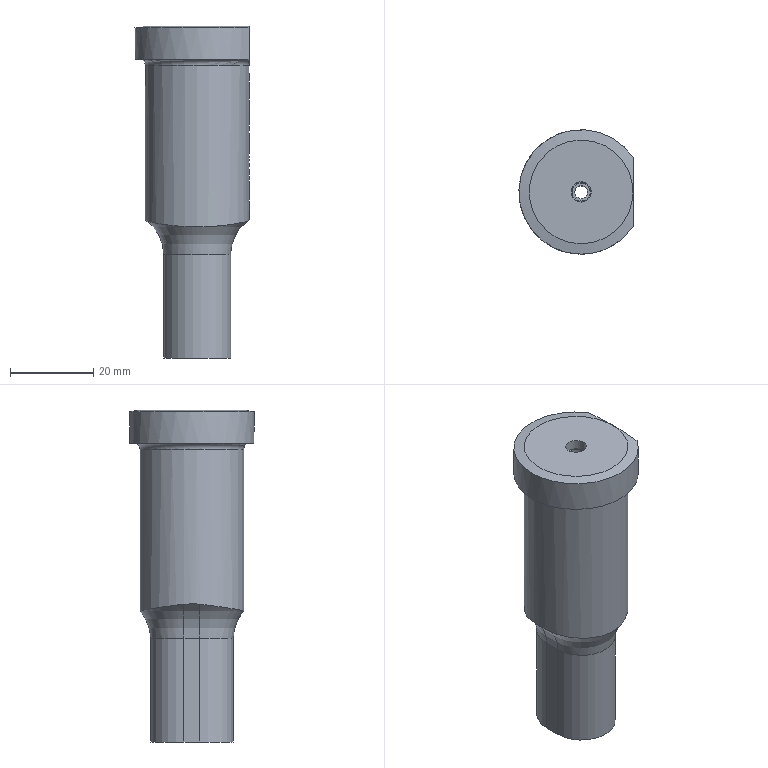Part | NX | features APJEL25-80-P20.00-W16.17_2 2 | 1 solid | 319 faces | box 27.501 x 30 x 80 mm | volume 33066 mm3 | plane 194 | cylinder 121 | torus 3 | cone 1 | commonest cylinder face diameters 24.8 x24 25 x11 0.87 x4 1.039 x4 1.042 x4 1.054 x4